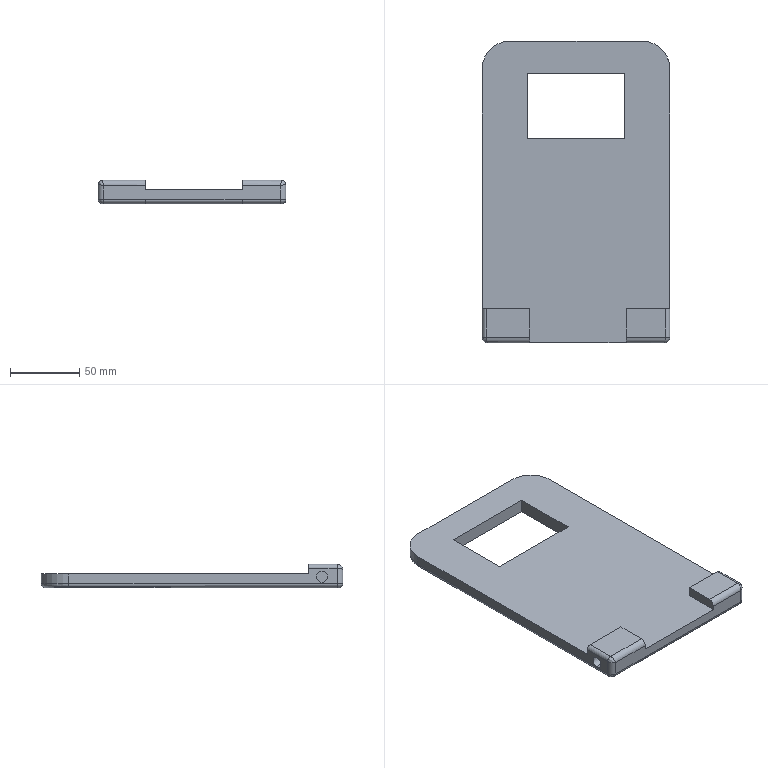Part | SolidWorks | features ICE 10, Fillet 6, Extrusion 1 | 1 solid | 787 faces | box 135.332 x 217.534 x 17 mm | volume 263326 mm3 | plane 554 | spline 211 | cylinder 18 | torus 4 | commonest cylinder face diameters 6 x8 8 x8 40 x2